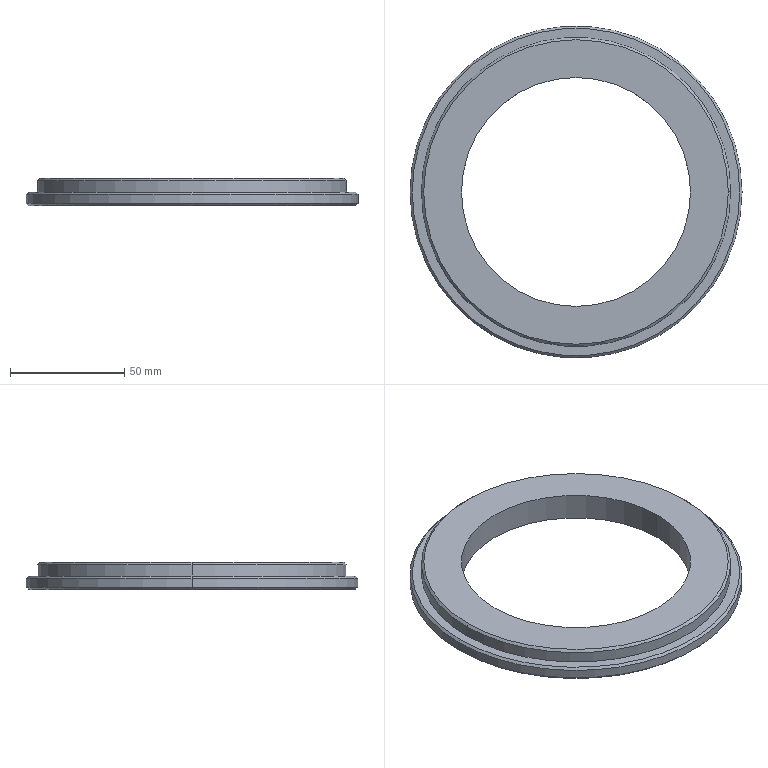Part | SolidWorks | features ICE 2, Chamfer 1, Extrusion 1, HoleWzd 1 | 1 solid | 39 faces | box 145 x 145 x 12 mm | volume 88157 mm3 | cylinder 18 | cone 18 | plane 3 | commonest cylinder face diameters 6.8 x12 100 x2 135 x2 145 x2
STEP:
#1=CARTESIAN_POINT('',(33.4,51.962,8.));
#2=VERTEX_POINT('',#1);
#3=CARTESIAN_POINT('',(26.6,51.962,8.));
#4=VERTEX_POINT('',#3);
#5=CARTESIAN_POINT('',(30.,51.962,8.));
#6=DIRECTION('',(0.,0.,-1.));
#7=DIRECTION('',(-1.,0.,0.));
#8=AXIS2_PLACEMENT_3D('',#5,#6,#7);
#9=CIRCLE('',#8,3.4);
#10=EDGE_CURVE('',#2,#4,#9,.T.);
#11=ORIENTED_EDGE('',*,*,#10,.F.);
#12=CARTESIAN_POINT('',(33.4,51.962,0.));
#13=VERTEX_POINT('',#12);
#14=CARTESIAN_POINT('',(33.4,51.962,0.));
#15=DIRECTION('',(0.,0.,-1.));
#16=VECTOR('',#15,1000.);
#17=LINE('',#14,#16);
#18=EDGE_CURVE('',#2,#13,#17,.T.);
#19=ORIENTED_EDGE('',*,*,#18,.T.);
#20=CARTESIAN_POINT('',(26.6,51.962,0.));
#21=VERTEX_POINT('',#20);
#22=CARTESIAN_POINT('',(30.,51.962,0.));
#23=DIRECTION('',(0.,0.,-1.));
#24=DIRECTION('',(-1.,0.,0.));
#25=AXIS2_PLACEMENT_3D('',#22,#23,#24);
#26=CIRCLE('',#25,3.4);
#27=EDGE_CURVE('',#13,#21,#26,.T.);
#28=ORIENTED_EDGE('',*,*,#27,.T.);
#29=CARTESIAN_POINT('',(26.6,51.962,0.));
#30=DIRECTION('',(0.,0.,-1.));
#31=VECTOR('',#30,1000.);
#32=LINE('',#29,#31);
#33=EDGE_CURVE('',#4,#21,#32,.T.);
#34=ORIENTED_EDGE('',*,*,#33,.F.);
#35=EDGE_LOOP('',(#11,#19,#28,#34));
#36=FACE_OUTER_BOUND('',#35,.T.);
#37=CARTESIAN_POINT('',(30.,51.962,0.));
#38=DIRECTION('',(0.,0.,-1.));
#39=DIRECTION('',(-1.,0.,0.));
#40=AXIS2_PLACEMENT_3D('',#37,#38,#39);
#41=CYLINDRICAL_SURFACE('',#40,3.4);
#42=ADVANCED_FACE('',(#36),#41,.F.);
#43=CARTESIAN_POINT('',(30.,51.962,10.043));
#44=VERTEX_POINT('',#43);
#45=CARTESIAN_POINT('',(26.6,51.962,8.));
#46=DIRECTION('',(-0.8572,0.,-0.515));
#47=VECTOR('',#46,1000.);
#48=LINE('',#45,#47);
#49=EDGE_CURVE('',#44,#4,#48,.T.);
#50=ORIENTED_EDGE('',*,*,#49,.F.);
#51=CARTESIAN_POINT('',(33.4,51.962,8.));
#52=DIRECTION('',(0.8572,0.,-0.515));
#53=VECTOR('',#52,1000.);
#54=LINE('',#51,#53);
#55=EDGE_CURVE('',#44,#2,#54,.T.);
#56=ORIENTED_EDGE('',*,*,#55,.T.);
#57=ORIENTED_EDGE('',*,*,#10,.T.);
#58=EDGE_LOOP('',(#50,#56,#57));
#59=FACE_OUTER_BOUND('',#58,.T.);
#60=CARTESIAN_POINT('',(30.,51.962,8.));
#61=DIRECTION('',(0.,0.,-1.));
#62=DIRECTION('',(-1.,0.,0.));
#63=AXIS2_PLACEMENT_3D('',#60,#61,#62);
#64=CONICAL_SURFACE('',#63,3.4,1.03);
#65=ADVANCED_FACE('',(#59),#64,.F.);
#66=CARTESIAN_POINT('',(-26.6,51.962,8.));
#67=VERTEX_POINT('',#66);
#68=CARTESIAN_POINT('',(-33.4,51.962,8.));
#69=VERTEX_POINT('',#68);
#70=CARTESIAN_POINT('',(-30.,51.962,8.));
#71=DIRECTION('',(0.,0.,-1.));
#72=DIRECTION('',(-1.,0.,0.));
#73=AXIS2_PLACEMENT_3D('',#70,#71,#72);
#74=CIRCLE('',#73,3.4);
#75=EDGE_CURVE('',#67,#69,#74,.T.);
#76=ORIENTED_EDGE('',*,*,#75,.F.);
#77=CARTESIAN_POINT('',(-26.6,51.962,0.));
#78=VERTEX_POINT('',#77);
#79=CARTESIAN_POINT('',(-26.6,51.962,0.));
#80=DIRECTION('',(0.,0.,-1.));
#81=VECTOR('',#80,1000.);
#82=LINE('',#79,#81);
#83=EDGE_CURVE('',#67,#78,#82,.T.);
#84=ORIENTED_EDGE('',*,*,#83,.T.);
#85=CARTESIAN_POINT('',(-33.4,51.962,0.));
#86=VERTEX_POINT('',#85);
#87=CARTESIAN_POINT('',(-30.,51.962,0.));
#88=DIRECTION('',(0.,0.,-1.));
#89=DIRECTION('',(-1.,0.,0.));
#90=AXIS2_PLACEMENT_3D('',#87,#88,#89);
#91=CIRCLE('',#90,3.4);
#92=EDGE_CURVE('',#78,#86,#91,.T.);
#93=ORIENTED_EDGE('',*,*,#92,.T.);
#94=CARTESIAN_POINT('',(-33.4,51.962,0.));
#95=DIRECTION('',(0.,0.,-1.));
#96=VECTOR('',#95,1000.);
#97=LINE('',#94,#96);
#98=EDGE_CURVE('',#69,#86,#97,.T.);
#99=ORIENTED_EDGE('',*,*,#98,.F.);
#100=EDGE_LOOP('',(#76,#84,#93,#99));
#101=FACE_OUTER_BOUND('',#100,.T.);
#102=CARTESIAN_POINT('',(-30.,51.962,0.));
#103=DIRECTION('',(0.,0.,-1.));
#104=DIRECTION('',(-1.,0.,0.));
#105=AXIS2_PLACEMENT_3D('',#102,#103,#104);
#106=CYLINDRICAL_SURFACE('',#105,3.4);
#107=ADVANCED_FACE('',(#101),#106,.F.);
#108=CARTESIAN_POINT('',(-30.,51.962,10.043));
#109=VERTEX_POINT('',#108);
#110=CARTESIAN_POINT('',(-33.4,51.962,8.));
#111=DIRECTION('',(-0.8572,0.,-0.515));
#112=VECTOR('',#111,1000.);
#113=LINE('',#110,#112);
#114=EDGE_CURVE('',#109,#69,#113,.T.);
#115=ORIENTED_EDGE('',*,*,#114,.F.);
#116=CARTESIAN_POINT('',(-26.6,51.962,8.));
#117=DIRECTION('',(0.8572,0.,-0.515));
#118=VECTOR('',#117,1000.);
#119=LINE('',#116,#118);
#120=EDGE_CURVE('',#109,#67,#119,.T.);
#121=ORIENTED_EDGE('',*,*,#120,.T.);
#122=ORIENTED_EDGE('',*,*,#75,.T.);
#123=EDGE_LOOP('',(#115,#121,#122));
#124=FACE_OUTER_BOUND('',#123,.T.);
#125=CARTESIAN_POINT('',(-30.,51.962,8.));
#126=DIRECTION('',(0.,0.,-1.));
#127=DIRECTION('',(-1.,0.,0.));
#128=AXIS2_PLACEMENT_3D('',#125,#126,#127);
#129=CONICAL_SURFACE('',#128,3.4,1.03);
#130=ADVANCED_FACE('',(#124),#129,.F.);
#131=CARTESIAN_POINT('',(-56.6,0.,8.));
#132=VERTEX_POINT('',#131);
#133=CARTESIAN_POINT('',(-63.4,0.,8.));
#134=VERTEX_POINT('',#133);
#135=CARTESIAN_POINT('',(-60.,0.,8.));
#136=DIRECTION('',(0.,0.,-1.));
#137=DIRECTION('',(-1.,0.,0.));
#138=AXIS2_PLACEMENT_3D('',#135,#136,#137);
#139=CIRCLE('',#138,3.4);
#140=EDGE_CURVE('',#132,#134,#139,.T.);
#141=ORIENTED_EDGE('',*,*,#140,.F.);
#142=CARTESIAN_POINT('',(-56.6,0.,0.));
#143=VERTEX_POINT('',#142);
#144=CARTESIAN_POINT('',(-56.6,0.,0.));
#145=DIRECTION('',(0.,0.,-1.));
#146=VECTOR('',#145,1000.);
#147=LINE('',#144,#146);
#148=EDGE_CURVE('',#132,#143,#147,.T.);
#149=ORIENTED_EDGE('',*,*,#148,.T.);
#150=CARTESIAN_POINT('',(-63.4,0.,0.));
#151=VERTEX_POINT('',#150);
#152=CARTESIAN_POINT('',(-60.,0.,0.));
#153=DIRECTION('',(0.,0.,-1.));
#154=DIRECTION('',(-1.,0.,0.));
#155=AXIS2_PLACEMENT_3D('',#152,#153,#154);
#156=CIRCLE('',#155,3.4);
#157=EDGE_CURVE('',#143,#151,#156,.T.);
#158=ORIENTED_EDGE('',*,*,#157,.T.);
#159=CARTESIAN_POINT('',(-63.4,0.,0.));
#160=DIRECTION('',(0.,0.,-1.));
#161=VECTOR('',#160,1000.);
#162=LINE('',#159,#161);
#163=EDGE_CURVE('',#134,#151,#162,.T.);
#164=ORIENTED_EDGE('',*,*,#163,.F.);
#165=EDGE_LOOP('',(#141,#149,#158,#164));
#166=FACE_OUTER_BOUND('',#165,.T.);
#167=CARTESIAN_POINT('',(-60.,0.,0.));
#168=DIRECTION('',(0.,0.,-1.));
#169=DIRECTION('',(-1.,0.,0.));
#170=AXIS2_PLACEMENT_3D('',#167,#168,#169);
#171=CYLINDRICAL_SURFACE('',#170,3.4);
#172=ADVANCED_FACE('',(#166),#171,.F.);
#173=CARTESIAN_POINT('',(-60.,0.,10.043));
#174=VERTEX_POINT('',#173);
#175=CARTESIAN_POINT('',(-63.4,0.,8.));
#176=DIRECTION('',(-0.8572,0.,-0.515));
#177=VECTOR('',#176,1000.);
#178=LINE('',#175,#177);
#179=EDGE_CURVE('',#174,#134,#178,.T.);
#180=ORIENTED_EDGE('',*,*,#179,.F.);
#181=CARTESIAN_POINT('',(-56.6,0.,8.));
#182=DIRECTION('',(0.8572,0.,-0.515));
#183=VECTOR('',#182,1000.);
#184=LINE('',#181,#183);
#185=EDGE_CURVE('',#174,#132,#184,.T.);
#186=ORIENTED_EDGE('',*,*,#185,.T.);
#187=ORIENTED_EDGE('',*,*,#140,.T.);
#188=EDGE_LOOP('',(#180,#186,#187));
#189=FACE_OUTER_BOUND('',#188,.T.);
#190=CARTESIAN_POINT('',(-60.,0.,8.));
#191=DIRECTION('',(0.,0.,-1.));
#192=DIRECTION('',(-1.,0.,0.));
#193=AXIS2_PLACEMENT_3D('',#190,#191,#192);
#194=CONICAL_SURFACE('',#193,3.4,1.03);
#195=ADVANCED_FACE('',(#189),#194,.F.);
#196=CARTESIAN_POINT('',(-26.6,-51.962,8.));
#197=VERTEX_POINT('',#196);
#198=CARTESIAN_POINT('',(-33.4,-51.962,8.));
#199=VERTEX_POINT('',#198);
#200=CARTESIAN_POINT('',(-30.,-51.962,8.));
#201=DIRECTION('',(0.,0.,-1.));
#202=DIRECTION('',(-1.,0.,0.));
#203=AXIS2_PLACEMENT_3D('',#200,#201,#202);
#204=CIRCLE('',#203,3.4);
#205=EDGE_CURVE('',#197,#199,#204,.T.);
#206=ORIENTED_EDGE('',*,*,#205,.F.);
#207=CARTESIAN_POINT('',(-26.6,-51.962,0.));
#208=VERTEX_POINT('',#207);
#209=CARTESIAN_POINT('',(-26.6,-51.962,0.));
#210=DIRECTION('',(0.,0.,-1.));
#211=VECTOR('',#210,1000.);
#212=LINE('',#209,#211);
#213=EDGE_CURVE('',#197,#208,#212,.T.);
#214=ORIENTED_EDGE('',*,*,#213,.T.);
#215=CARTESIAN_POINT('',(-33.4,-51.962,0.));
#216=VERTEX_POINT('',#215);
#217=CARTESIAN_POINT('',(-30.,-51.962,0.));
#218=DIRECTION('',(0.,0.,-1.));
#219=DIRECTION('',(-1.,0.,0.));
#220=AXIS2_PLACEMENT_3D('',#217,#218,#219);
#221=CIRCLE('',#220,3.4);
#222=EDGE_CURVE('',#208,#216,#221,.T.);
#223=ORIENTED_EDGE('',*,*,#222,.T.);
#224=CARTESIAN_POINT('',(-33.4,-51.962,0.));
#225=DIRECTION('',(0.,0.,-1.));
#226=VECTOR('',#225,1000.);
#227=LINE('',#224,#226);
#228=EDGE_CURVE('',#199,#216,#227,.T.);
#229=ORIENTED_EDGE('',*,*,#228,.F.);
#230=EDGE_LOOP('',(#206,#214,#223,#229));
#231=FACE_OUTER_BOUND('',#230,.T.);
#232=CARTESIAN_POINT('',(-30.,-51.962,0.));
#233=DIRECTION('',(0.,0.,-1.));
#234=DIRECTION('',(-1.,0.,0.));
#235=AXIS2_PLACEMENT_3D('',#232,#233,#234);
#236=CYLINDRICAL_SURFACE('',#235,3.4);
#237=ADVANCED_FACE('',(#231),#236,.F.);
#238=CARTESIAN_POINT('',(-30.,-51.962,10.043));
#239=VERTEX_POINT('',#238);
#240=CARTESIAN_POINT('',(-33.4,-51.962,8.));
#241=DIRECTION('',(-0.8572,0.,-0.515));
#242=VECTOR('',#241,1000.);
#243=LINE('',#240,#242);
#244=EDGE_CURVE('',#239,#199,#243,.T.);
#245=ORIENTED_EDGE('',*,*,#244,.F.);
#246=CARTESIAN_POINT('',(-26.6,-51.962,8.));
#247=DIRECTION('',(0.8572,0.,-0.515));
#248=VECTOR('',#247,1000.);
#249=LINE('',#246,#248);
#250=EDGE_CURVE('',#239,#197,#249,.T.);
#251=ORIENTED_EDGE('',*,*,#250,.T.);
#252=ORIENTED_EDGE('',*,*,#205,.T.);
#253=EDGE_LOOP('',(#245,#251,#252));
#254=FACE_OUTER_BOUND('',#253,.T.);
#255=CARTESIAN_POINT('',(-30.,-51.962,8.));
#256=DIRECTION('',(0.,0.,-1.));
#257=DIRECTION('',(-1.,0.,0.));
#258=AXIS2_PLACEMENT_3D('',#255,#256,#257);
#259=CONICAL_SURFACE('',#258,3.4,1.03);
#260=ADVANCED_FACE('',(#254),#259,.F.);
#261=CARTESIAN_POINT('',(33.4,-51.962,8.));
#262=VERTEX_POINT('',#261);
#263=CARTESIAN_POINT('',(26.6,-51.962,8.));
#264=VERTEX_POINT('',#263);
#265=CARTESIAN_POINT('',(30.,-51.962,8.));
#266=DIRECTION('',(0.,0.,-1.));
#267=DIRECTION('',(-1.,0.,0.));
#268=AXIS2_PLACEMENT_3D('',#265,#266,#267);
#269=CIRCLE('',#268,3.4);
#270=EDGE_CURVE('',#262,#264,#269,.T.);
#271=ORIENTED_EDGE('',*,*,#270,.F.);
#272=CARTESIAN_POINT('',(33.4,-51.962,0.));
#273=VERTEX_POINT('',#272);
#274=CARTESIAN_POINT('',(33.4,-51.962,0.));
#275=DIRECTION('',(0.,0.,-1.));
#276=VECTOR('',#275,1000.);
#277=LINE('',#274,#276);
#278=EDGE_CURVE('',#262,#273,#277,.T.);
#279=ORIENTED_EDGE('',*,*,#278,.T.);
#280=CARTESIAN_POINT('',(26.6,-51.962,0.));
#281=VERTEX_POINT('',#280);
#282=CARTESIAN_POINT('',(30.,-51.962,0.));
#283=DIRECTION('',(0.,0.,-1.));
#284=DIRECTION('',(-1.,0.,0.));
#285=AXIS2_PLACEMENT_3D('',#282,#283,#284);
#286=CIRCLE('',#285,3.4);
#287=EDGE_CURVE('',#273,#281,#286,.T.);
#288=ORIENTED_EDGE('',*,*,#287,.T.);
#289=CARTESIAN_POINT('',(26.6,-51.962,0.));
#290=DIRECTION('',(0.,0.,-1.));
#291=VECTOR('',#290,1000.);
#292=LINE('',#289,#291);
#293=EDGE_CURVE('',#264,#281,#292,.T.);
#294=ORIENTED_EDGE('',*,*,#293,.F.);
#295=EDGE_LOOP('',(#271,#279,#288,#294));
#296=FACE_OUTER_BOUND('',#295,.T.);
#297=CARTESIAN_POINT('',(30.,-51.962,0.));
#298=DIRECTION('',(0.,0.,-1.));
#299=DIRECTION('',(-1.,0.,0.));
#300=AXIS2_PLACEMENT_3D('',#297,#298,#299);
#301=CYLINDRICAL_SURFACE('',#300,3.4);
#302=ADVANCED_FACE('',(#296),#301,.F.);
#303=CARTESIAN_POINT('',(30.,-51.962,10.043));
#304=VERTEX_POINT('',#303);
#305=CARTESIAN_POINT('',(26.6,-51.962,8.));
#306=DIRECTION('',(-0.8572,0.,-0.515));
#307=VECTOR('',#306,1000.);
#308=LINE('',#305,#307);
#309=EDGE_CURVE('',#304,#264,#308,.T.);
#310=ORIENTED_EDGE('',*,*,#309,.F.);
#311=CARTESIAN_POINT('',(33.4,-51.962,8.));
#312=DIRECTION('',(0.8572,0.,-0.515));
#313=VECTOR('',#312,1000.);
#314=LINE('',#311,#313);
#315=EDGE_CURVE('',#304,#262,#314,.T.);
#316=ORIENTED_EDGE('',*,*,#315,.T.);
#317=ORIENTED_EDGE('',*,*,#270,.T.);
#318=EDGE_LOOP('',(#310,#316,#317));
#319=FACE_OUTER_BOUND('',#318,.T.);
#320=CARTESIAN_POINT('',(30.,-51.962,8.));
#321=DIRECTION('',(0.,0.,-1.));
#322=DIRECTION('',(-1.,0.,0.));
#323=AXIS2_PLACEMENT_3D('',#320,#321,#322);
#324=CONICAL_SURFACE('',#323,3.4,1.03);
#325=ADVANCED_FACE('',(#319),#324,.F.);
#326=CARTESIAN_POINT('',(63.4,0.,8.));
#327=VERTEX_POINT('',#326);
#328=CARTESIAN_POINT('',(56.6,0.,8.));
#329=VERTEX_POINT('',#328);
#330=CARTESIAN_POINT('',(60.,0.,8.));
#331=DIRECTION('',(0.,0.,-1.));
#332=DIRECTION('',(-1.,0.,0.));
#333=AXIS2_PLACEMENT_3D('',#330,#331,#332);
#334=CIRCLE('',#333,3.4);
#335=EDGE_CURVE('',#327,#329,#334,.T.);
#336=ORIENTED_EDGE('',*,*,#335,.F.);
#337=CARTESIAN_POINT('',(63.4,0.,0.));
#338=VERTEX_POINT('',#337);
#339=CARTESIAN_POINT('',(63.4,0.,0.));
#340=DIRECTION('',(0.,0.,-1.));
#341=VECTOR('',#340,1000.);
#342=LINE('',#339,#341);
#343=EDGE_CURVE('',#327,#338,#342,.T.);
#344=ORIENTED_EDGE('',*,*,#343,.T.);
#345=CARTESIAN_POINT('',(56.6,0.,0.));
#346=VERTEX_POINT('',#345);
#347=CARTESIAN_POINT('',(60.,0.,0.));
#348=DIRECTION('',(0.,0.,-1.));
#349=DIRECTION('',(-1.,0.,0.));
#350=AXIS2_PLACEMENT_3D('',#347,#348,#349);
#351=CIRCLE('',#350,3.4);
#352=EDGE_CURVE('',#338,#346,#351,.T.);
#353=ORIENTED_EDGE('',*,*,#352,.T.);
#354=CARTESIAN_POINT('',(56.6,0.,0.));
#355=DIRECTION('',(0.,0.,-1.));
#356=VECTOR('',#355,1000.);
#357=LINE('',#354,#356);
#358=EDGE_CURVE('',#329,#346,#357,.T.);
#359=ORIENTED_EDGE('',*,*,#358,.F.);
#360=EDGE_LOOP('',(#336,#344,#353,#359));
#361=FACE_OUTER_BOUND('',#360,.T.);
#362=CARTESIAN_POINT('',(60.,0.,0.));
#363=DIRECTION('',(0.,0.,-1.));
#364=DIRECTION('',(-1.,0.,0.));
#365=AXIS2_PLACEMENT_3D('',#362,#363,#364);
#366=CYLINDRICAL_SURFACE('',#365,3.4);
#367=ADVANCED_FACE('',(#361),#366,.F.);
#368=CARTESIAN_POINT('',(60.,0.,10.043));
#369=VERTEX_POINT('',#368);
#370=CARTESIAN_POINT('',(56.6,0.,8.));
#371=DIRECTION('',(-0.8572,0.,-0.515));
#372=VECTOR('',#371,1000.);
#373=LINE('',#370,#372);
#374=EDGE_CURVE('',#369,#329,#373,.T.);
#375=ORIENTED_EDGE('',*,*,#374,.F.);
#376=CARTESIAN_POINT('',(63.4,0.,8.));
#377=DIRECTION('',(0.8572,0.,-0.515));
#378=VECTOR('',#377,1000.);
#379=LINE('',#376,#378);
#380=EDGE_CURVE('',#369,#327,#379,.T.);
#381=ORIENTED_EDGE('',*,*,#380,.T.);
#382=ORIENTED_EDGE('',*,*,#335,.T.);
#383=EDGE_LOOP('',(#375,#381,#382));
#384=FACE_OUTER_BOUND('',#383,.T.);
#385=CARTESIAN_POINT('',(60.,0.,8.));
#386=DIRECTION('',(0.,0.,-1.));
#387=DIRECTION('',(-1.,0.,0.));
#388=AXIS2_PLACEMENT_3D('',#385,#386,#387);
#389=CONICAL_SURFACE('',#388,3.4,1.03);
#390=ADVANCED_FACE('',(#384),#389,.F.);
#391=CARTESIAN_POINT('',(-71.5,0.,0.));
#392=VERTEX_POINT('',#391);
#393=CARTESIAN_POINT('',(71.5,0.,0.));
#394=VERTEX_POINT('',#393);
#395=CARTESIAN_POINT('',(0.,0.,0.));
#396=DIRECTION('',(0.,0.,-1.));
#397=DIRECTION('',(1.,0.,0.));
#398=AXIS2_PLACEMENT_3D('',#395,#396,#397);
#399=CIRCLE('',#398,71.5);
#400=EDGE_CURVE('',#392,#394,#399,.T.);
#401=ORIENTED_EDGE('',*,*,#400,.F.);
#402=CARTESIAN_POINT('',(-72.5,0.,1.));
#403=VERTEX_POINT('',#402);
#404=CARTESIAN_POINT('',(-72.5,0.,1.));
#405=DIRECTION('',(-0.7071,0.,0.7071));
#406=VECTOR('',#405,1000.);
#407=LINE('',#404,#406);
#408=EDGE_CURVE('',#392,#403,#407,.T.);
#409=ORIENTED_EDGE('',*,*,#408,.T.);
#410=CARTESIAN_POINT('',(72.5,0.,1.));
#411=VERTEX_POINT('',#410);
#412=CARTESIAN_POINT('',(0.,0.,1.));
#413=DIRECTION('',(0.,0.,1.));
#414=DIRECTION('',(1.,0.,0.));
#415=AXIS2_PLACEMENT_3D('',#412,#413,#414);
#416=CIRCLE('',#415,72.5);
#417=EDGE_CURVE('',#411,#403,#416,.T.);
#418=ORIENTED_EDGE('',*,*,#417,.F.);
#419=CARTESIAN_POINT('',(72.5,0.,1.));
#420=DIRECTION('',(0.7071,0.,0.7071));
#421=VECTOR('',#420,1000.);
#422=LINE('',#419,#421);
#423=EDGE_CURVE('',#394,#411,#422,.T.);
#424=ORIENTED_EDGE('',*,*,#423,.F.);
#425=EDGE_LOOP('',(#401,#409,#418,#424));
#426=FACE_OUTER_BOUND('',#425,.T.);
#427=CARTESIAN_POINT('',(0.,0.,1.));
#428=DIRECTION('',(0.,0.,1.));
#429=DIRECTION('',(1.,0.,0.));
#430=AXIS2_PLACEMENT_3D('',#427,#428,#429);
#431=CONICAL_SURFACE('',#430,72.5,0.7854);
#432=ADVANCED_FACE('',(#426),#431,.T.);
#433=CARTESIAN_POINT('',(71.5,0.,6.));
#434=VERTEX_POINT('',#433);
#435=CARTESIAN_POINT('',(-71.5,0.,6.));
#436=VERTEX_POINT('',#435);
#437=CARTESIAN_POINT('',(0.,0.,6.));
#438=DIRECTION('',(0.,0.,1.));
#439=DIRECTION('',(1.,0.,0.));
#440=AXIS2_PLACEMENT_3D('',#437,#438,#439);
#441=CIRCLE('',#440,71.5);
#442=EDGE_CURVE('',#434,#436,#441,.T.);
#443=ORIENTED_EDGE('',*,*,#442,.F.);
#444=CARTESIAN_POINT('',(72.5,0.,5.));
#445=VERTEX_POINT('',#444);
#446=CARTESIAN_POINT('',(71.5,0.,6.));
#447=DIRECTION('',(0.7071,0.,-0.7071));
#448=VECTOR('',#447,1000.);
#449=LINE('',#446,#448);
#450=EDGE_CURVE('',#434,#445,#449,.T.);
#451=ORIENTED_EDGE('',*,*,#450,.T.);
#452=CARTESIAN_POINT('',(-72.5,0.,5.));
#453=VERTEX_POINT('',#452);
#454=CARTESIAN_POINT('',(0.,0.,5.));
#455=DIRECTION('',(0.,0.,-1.));
#456=DIRECTION('',(1.,0.,0.));
#457=AXIS2_PLACEMENT_3D('',#454,#455,#456);
#458=CIRCLE('',#457,72.5);
#459=EDGE_CURVE('',#453,#445,#458,.T.);
#460=ORIENTED_EDGE('',*,*,#459,.F.);
#461=CARTESIAN_POINT('',(-71.5,0.,6.));
#462=DIRECTION('',(-0.7071,0.,-0.7071));
#463=VECTOR('',#462,1000.);
#464=LINE('',#461,#463);
#465=EDGE_CURVE('',#436,#453,#464,.T.);
#466=ORIENTED_EDGE('',*,*,#465,.F.);
#467=EDGE_LOOP('',(#443,#451,#460,#466));
#468=FACE_OUTER_BOUND('',#467,.T.);
#469=CARTESIAN_POINT('',(0.,0.,6.));
#470=DIRECTION('',(0.,0.,-1.));
#471=DIRECTION('',(-1.,0.,0.));
#472=AXIS2_PLACEMENT_3D('',#469,#470,#471);
#473=CONICAL_SURFACE('',#472,71.5,0.7854);
#474=ADVANCED_FACE('',(#468),#473,.T.);
#475=CARTESIAN_POINT('',(66.5,0.,12.));
#476=VERTEX_POINT('',#475);
#477=CARTESIAN_POINT('',(-66.5,0.,12.));
#478=VERTEX_POINT('',#477);
#479=CARTESIAN_POINT('',(0.,0.,12.));
#480=DIRECTION('',(0.,0.,1.));
#481=DIRECTION('',(1.,0.,0.));
#482=AXIS2_PLACEMENT_3D('',#479,#480,#481);
#483=CIRCLE('',#482,66.5);
#484=EDGE_CURVE('',#476,#478,#483,.T.);
#485=ORIENTED_EDGE('',*,*,#484,.F.);
#486=CARTESIAN_POINT('',(67.5,0.,11.));
#487=VERTEX_POINT('',#486);
#488=CARTESIAN_POINT('',(66.5,0.,12.));
#489=DIRECTION('',(0.7071,0.,-0.7071));
#490=VECTOR('',#489,1000.);
#491=LINE('',#488,#490);
#492=EDGE_CURVE('',#476,#487,#491,.T.);
#493=ORIENTED_EDGE('',*,*,#492,.T.);
#494=CARTESIAN_POINT('',(-67.5,0.,11.));
#495=VERTEX_POINT('',#494);
#496=CARTESIAN_POINT('',(0.,0.,11.));
#497=DIRECTION('',(0.,0.,-1.));
#498=DIRECTION('',(1.,0.,0.));
#499=AXIS2_PLACEMENT_3D('',#496,#497,#498);
#500=CIRCLE('',#499,67.5);
#501=EDGE_CURVE('',#495,#487,#500,.T.);
#502=ORIENTED_EDGE('',*,*,#501,.F.);
#503=CARTESIAN_POINT('',(-66.5,0.,12.));
#504=DIRECTION('',(-0.7071,0.,-0.7071));
#505=VECTOR('',#504,1000.);
#506=LINE('',#503,#505);
#507=EDGE_CURVE('',#478,#495,#506,.T.);
#508=ORIENTED_EDGE('',*,*,#507,.F.);
#509=EDGE_LOOP('',(#485,#493,#502,#508));
#510=FACE_OUTER_BOUND('',#509,.T.);
#511=CARTESIAN_POINT('',(0.,0.,12.));
#512=DIRECTION('',(0.,0.,-1.));
#513=DIRECTION('',(-1.,0.,0.));
#514=AXIS2_PLACEMENT_3D('',#511,#512,#513);
#515=CONICAL_SURFACE('',#514,66.5,0.7854);
#516=ADVANCED_FACE('',(#510),#515,.T.);
#517=ORIENTED_EDGE('',*,*,#501,.T.);
#518=CARTESIAN_POINT('',(67.5,0.,6.));
#519=VERTEX_POINT('',#518);
#520=CARTESIAN_POINT('',(67.5,0.,12.));
#521=DIRECTION('',(0.,0.,-1.));
#522=VECTOR('',#521,1000.);
#523=LINE('',#520,#522);
#524=EDGE_CURVE('',#487,#519,#523,.T.);
#525=ORIENTED_EDGE('',*,*,#524,.T.);
#526=CARTESIAN_POINT('',(-67.5,0.,6.));
#527=VERTEX_POINT('',#526);
#528=CARTESIAN_POINT('',(0.,0.,6.));
#529=DIRECTION('',(0.,0.,1.));
#530=DIRECTION('',(1.,0.,0.));
#531=AXIS2_PLACEMENT_3D('',#528,#529,#530);
#532=CIRCLE('',#531,67.5);
#533=EDGE_CURVE('',#519,#527,#532,.T.);
#534=ORIENTED_EDGE('',*,*,#533,.T.);
#535=CARTESIAN_POINT('',(-67.5,0.,12.));
#536=DIRECTION('',(0.,0.,-1.));
#537=VECTOR('',#536,1000.);
#538=LINE('',#535,#537);
#539=EDGE_CURVE('',#495,#527,#538,.T.);
#540=ORIENTED_EDGE('',*,*,#539,.F.);
#541=EDGE_LOOP('',(#517,#525,#534,#540));
#542=FACE_OUTER_BOUND('',#541,.T.);
#543=CARTESIAN_POINT('',(0.,0.,12.));
#544=DIRECTION('',(0.,0.,-1.));
#545=DIRECTION('',(-1.,0.,0.));
#546=AXIS2_PLACEMENT_3D('',#543,#544,#545);
#547=CYLINDRICAL_SURFACE('',#546,67.5);
#548=ADVANCED_FACE('',(#542),#547,.T.);
#549=CARTESIAN_POINT('',(-50.,0.,12.));
#550=VERTEX_POINT('',#549);
#551=CARTESIAN_POINT('',(50.,0.,12.));
#552=VERTEX_POINT('',#551);
#553=CARTESIAN_POINT('',(0.,0.,12.));
#554=DIRECTION('',(0.,0.,1.));
#555=DIRECTION('',(1.,0.,0.));
#556=AXIS2_PLACEMENT_3D('',#553,#554,#555);
#557=CIRCLE('',#556,50.);
#558=EDGE_CURVE('',#550,#552,#557,.T.);
#559=ORIENTED_EDGE('',*,*,#558,.T.);
#560=CARTESIAN_POINT('',(50.,0.,0.));
#561=VERTEX_POINT('',#560);
#562=CARTESIAN_POINT('',(50.,0.,6.));
#563=DIRECTION('',(0.,0.,-1.));
#564=VECTOR('',#563,1000.);
#565=LINE('',#562,#564);
#566=EDGE_CURVE('',#552,#561,#565,.T.);
#567=ORIENTED_EDGE('',*,*,#566,.T.);
#568=CARTESIAN_POINT('',(-50.,0.,0.));
#569=VERTEX_POINT('',#568);
#570=CARTESIAN_POINT('',(0.,0.,0.));
#571=DIRECTION('',(0.,0.,1.));
#572=DIRECTION('',(1.,0.,0.));
#573=AXIS2_PLACEMENT_3D('',#570,#571,#572);
#574=CIRCLE('',#573,50.);
#575=EDGE_CURVE('',#569,#561,#574,.T.);
#576=ORIENTED_EDGE('',*,*,#575,.F.);
#577=CARTESIAN_POINT('',(-50.,0.,6.));
#578=DIRECTION('',(0.,0.,-1.));
#579=VECTOR('',#578,1000.);
#580=LINE('',#577,#579);
#581=EDGE_CURVE('',#550,#569,#580,.T.);
#582=ORIENTED_EDGE('',*,*,#581,.F.);
#583=EDGE_LOOP('',(#559,#567,#576,#582));
#584=FACE_OUTER_BOUND('',#583,.T.);
#585=CARTESIAN_POINT('',(0.,0.,6.));
#586=DIRECTION('',(0.,0.,-1.));
#587=DIRECTION('',(-1.,0.,0.));
#588=AXIS2_PLACEMENT_3D('',#585,#586,#587);
#589=CYLINDRICAL_SURFACE('',#588,50.);
#590=ADVANCED_FACE('',(#584),#589,.F.);
#591=ORIENTED_EDGE('',*,*,#459,.T.);
#592=CARTESIAN_POINT('',(72.5,0.,6.));
#593=DIRECTION('',(0.,0.,-1.));
#594=VECTOR('',#593,1000.);
#595=LINE('',#592,#594);
#596=EDGE_CURVE('',#445,#411,#595,.T.);
#597=ORIENTED_EDGE('',*,*,#596,.T.);
#598=ORIENTED_EDGE('',*,*,#417,.T.);
#599=CARTESIAN_POINT('',(-72.5,0.,6.));
#600=DIRECTION('',(0.,0.,-1.));
#601=VECTOR('',#600,1000.);
#602=LINE('',#599,#601);
#603=EDGE_CURVE('',#453,#403,#602,.T.);
#604=ORIENTED_EDGE('',*,*,#603,.F.);
#605=EDGE_LOOP('',(#591,#597,#598,#604));
#606=FACE_OUTER_BOUND('',#605,.T.);
#607=CARTESIAN_POINT('',(0.,0.,6.));
#608=DIRECTION('',(0.,0.,-1.));
#609=DIRECTION('',(-1.,0.,0.));
#610=AXIS2_PLACEMENT_3D('',#607,#608,#609);
#611=CYLINDRICAL_SURFACE('',#610,72.5);
#612=ADVANCED_FACE('',(#606),#611,.T.);
#613=CARTESIAN_POINT('',(0.,0.,6.));
#614=DIRECTION('',(0.,0.,1.));
#615=DIRECTION('',(1.,0.,0.));
#616=AXIS2_PLACEMENT_3D('',#613,#614,#615);
#617=CIRCLE('',#616,71.5);
#618=EDGE_CURVE('',#436,#434,#617,.T.);
#619=ORIENTED_EDGE('',*,*,#618,.T.);
#620=ORIENTED_EDGE('',*,*,#442,.T.);
#621=EDGE_LOOP('',(#619,#620));
#622=FACE_OUTER_BOUND('',#621,.T.);
#623=CARTESIAN_POINT('',(0.,0.,6.));
#624=DIRECTION('',(0.,0.,1.));
#625=DIRECTION('',(1.,0.,0.));
#626=AXIS2_PLACEMENT_3D('',#623,#624,#625);
#627=CIRCLE('',#626,67.5);
#628=EDGE_CURVE('',#527,#519,#627,.T.);
#629=ORIENTED_EDGE('',*,*,#628,.F.);
#630=ORIENTED_EDGE('',*,*,#533,.F.);
#631=EDGE_LOOP('',(#629,#630));
#632=FACE_BOUND('',#631,.T.);
#633=CARTESIAN_POINT('',(0.,0.,6.));
#634=DIRECTION('',(0.,0.,1.));
#635=DIRECTION('',(1.,0.,0.));
#636=AXIS2_PLACEMENT_3D('',#633,#634,#635);
#637=PLANE('',#636);
#638=ADVANCED_FACE('',(#622,#632),#637,.T.);
#639=CARTESIAN_POINT('',(30.,51.962,0.));
#640=DIRECTION('',(0.,0.,-1.));
#641=DIRECTION('',(-1.,0.,0.));
#642=AXIS2_PLACEMENT_3D('',#639,#640,#641);
#643=CIRCLE('',#642,3.4);
#644=EDGE_CURVE('',#21,#13,#643,.T.);
#645=ORIENTED_EDGE('',*,*,#644,.F.);
#646=ORIENTED_EDGE('',*,*,#27,.F.);
#647=EDGE_LOOP('',(#645,#646));
#648=FACE_BOUND('',#647,.T.);
#649=CARTESIAN_POINT('',(-30.,51.962,0.));
#650=DIRECTION('',(0.,0.,-1.));
#651=DIRECTION('',(-1.,0.,0.));
#652=AXIS2_PLACEMENT_3D('',#649,#650,#651);
#653=CIRCLE('',#652,3.4);
#654=EDGE_CURVE('',#86,#78,#653,.T.);
#655=ORIENTED_EDGE('',*,*,#654,.F.);
#656=ORIENTED_EDGE('',*,*,#92,.F.);
#657=EDGE_LOOP('',(#655,#656));
#658=FACE_BOUND('',#657,.T.);
#659=CARTESIAN_POINT('',(-60.,0.,0.));
#660=DIRECTION('',(0.,0.,-1.));
#661=DIRECTION('',(-1.,0.,0.));
#662=AXIS2_PLACEMENT_3D('',#659,#660,#661);
#663=CIRCLE('',#662,3.4);
#664=EDGE_CURVE('',#151,#143,#663,.T.);
#665=ORIENTED_EDGE('',*,*,#664,.F.);
#666=ORIENTED_EDGE('',*,*,#157,.F.);
#667=EDGE_LOOP('',(#665,#666));
#668=FACE_BOUND('',#667,.T.);
#669=CARTESIAN_POINT('',(-30.,-51.962,0.));
#670=DIRECTION('',(0.,0.,-1.));
#671=DIRECTION('',(-1.,0.,0.));
#672=AXIS2_PLACEMENT_3D('',#669,#670,#671);
#673=CIRCLE('',#672,3.4);
#674=EDGE_CURVE('',#216,#208,#673,.T.);
#675=ORIENTED_EDGE('',*,*,#674,.F.);
#676=ORIENTED_EDGE('',*,*,#222,.F.);
#677=EDGE_LOOP('',(#675,#676));
#678=FACE_BOUND('',#677,.T.);
#679=CARTESIAN_POINT('',(30.,-51.962,0.));
#680=DIRECTION('',(0.,0.,-1.));
#681=DIRECTION('',(-1.,0.,0.));
#682=AXIS2_PLACEMENT_3D('',#679,#680,#681);
#683=CIRCLE('',#682,3.4);
#684=EDGE_CURVE('',#281,#273,#683,.T.);
#685=ORIENTED_EDGE('',*,*,#684,.F.);
#686=ORIENTED_EDGE('',*,*,#287,.F.);
#687=EDGE_LOOP('',(#685,#686));
#688=FACE_BOUND('',#687,.T.);
#689=CARTESIAN_POINT('',(60.,0.,0.));
#690=DIRECTION('',(0.,0.,-1.));
#691=DIRECTION('',(-1.,0.,0.));
#692=AXIS2_PLACEMENT_3D('',#689,#690,#691);
#693=CIRCLE('',#692,3.4);
#694=EDGE_CURVE('',#346,#338,#693,.T.);
#695=ORIENTED_EDGE('',*,*,#694,.F.);
#696=ORIENTED_EDGE('',*,*,#352,.F.);
#697=EDGE_LOOP('',(#695,#696));
#698=FACE_BOUND('',#697,.T.);
#699=CARTESIAN_POINT('',(0.,0.,0.));
#700=DIRECTION('',(0.,0.,-1.));
#701=DIRECTION('',(1.,0.,0.));
#702=AXIS2_PLACEMENT_3D('',#699,#700,#701);
#703=CIRCLE('',#702,71.5);
#704=EDGE_CURVE('',#394,#392,#703,.T.);
#705=ORIENTED_EDGE('',*,*,#704,.T.);
#706=ORIENTED_EDGE('',*,*,#400,.T.);
#707=EDGE_LOOP('',(#705,#706));
#708=FACE_OUTER_BOUND('',#707,.T.);
#709=ORIENTED_EDGE('',*,*,#575,.T.);
#710=CARTESIAN_POINT('',(0.,0.,0.));
#711=DIRECTION('',(0.,0.,1.));
#712=DIRECTION('',(1.,0.,0.));
#713=AXIS2_PLACEMENT_3D('',#710,#711,#712);
#714=CIRCLE('',#713,50.);
#715=EDGE_CURVE('',#561,#569,#714,.T.);
#716=ORIENTED_EDGE('',*,*,#715,.T.);
#717=EDGE_LOOP('',(#709,#716));
#718=FACE_BOUND('',#717,.T.);
#719=CARTESIAN_POINT('',(0.,0.,0.));
#720=DIRECTION('',(0.,0.,1.));
#721=DIRECTION('',(1.,0.,0.));
#722=AXIS2_PLACEMENT_3D('',#719,#720,#721);
#723=PLANE('',#722);
#724=ADVANCED_FACE('',(#648,#658,#668,#678,#688,#698,#708,#718),#723,.F.);
#725=ORIENTED_EDGE('',*,*,#596,.F.);
#726=CARTESIAN_POINT('',(0.,0.,5.));
#727=DIRECTION('',(0.,0.,-1.));
#728=DIRECTION('',(1.,0.,0.));
#729=AXIS2_PLACEMENT_3D('',#726,#727,#728);
#730=CIRCLE('',#729,72.5);
#731=EDGE_CURVE('',#445,#453,#730,.T.);
#732=ORIENTED_EDGE('',*,*,#731,.T.);
#733=ORIENTED_EDGE('',*,*,#603,.T.);
#734=CARTESIAN_POINT('',(0.,0.,1.));
#735=DIRECTION('',(0.,0.,1.));
#736=DIRECTION('',(1.,0.,0.));
#737=AXIS2_PLACEMENT_3D('',#734,#735,#736);
#738=CIRCLE('',#737,72.5);
#739=EDGE_CURVE('',#403,#411,#738,.T.);
#740=ORIENTED_EDGE('',*,*,#739,.T.);
#741=EDGE_LOOP('',(#725,#732,#733,#740));
#742=FACE_OUTER_BOUND('',#741,.T.);
#743=CARTESIAN_POINT('',(0.,0.,6.));
#744=DIRECTION('',(0.,0.,-1.));
#745=DIRECTION('',(-1.,0.,0.));
#746=AXIS2_PLACEMENT_3D('',#743,#744,#745);
#747=CYLINDRICAL_SURFACE('',#746,72.5);
#748=ADVANCED_FACE('',(#742),#747,.T.);
#749=ORIENTED_EDGE('',*,*,#566,.F.);
#750=CARTESIAN_POINT('',(0.,0.,12.));
#751=DIRECTION('',(0.,0.,1.));
#752=DIRECTION('',(1.,0.,0.));
#753=AXIS2_PLACEMENT_3D('',#750,#751,#752);
#754=CIRCLE('',#753,50.);
#755=EDGE_CURVE('',#552,#550,#754,.T.);
#756=ORIENTED_EDGE('',*,*,#755,.T.);
#757=ORIENTED_EDGE('',*,*,#581,.T.);
#758=ORIENTED_EDGE('',*,*,#715,.F.);
#759=EDGE_LOOP('',(#749,#756,#757,#758));
#760=FACE_OUTER_BOUND('',#759,.T.);
#761=CARTESIAN_POINT('',(0.,0.,6.));
#762=DIRECTION('',(0.,0.,-1.));
#763=DIRECTION('',(-1.,0.,0.));
#764=AXIS2_PLACEMENT_3D('',#761,#762,#763);
#765=CYLINDRICAL_SURFACE('',#764,50.);
#766=ADVANCED_FACE('',(#760),#765,.F.);
#767=CARTESIAN_POINT('',(0.,0.,12.));
#768=DIRECTION('',(0.,0.,1.));
#769=DIRECTION('',(1.,0.,0.));
#770=AXIS2_PLACEMENT_3D('',#767,#768,#769);
#771=CIRCLE('',#770,66.5);
#772=EDGE_CURVE('',#478,#476,#771,.T.);
#773=ORIENTED_EDGE('',*,*,#772,.T.);
#774=ORIENTED_EDGE('',*,*,#484,.T.);
#775=EDGE_LOOP('',(#773,#774));
#776=FACE_OUTER_BOUND('',#775,.T.);
#777=ORIENTED_EDGE('',*,*,#558,.F.);
#778=ORIENTED_EDGE('',*,*,#755,.F.);
#779=EDGE_LOOP('',(#777,#778));
#780=FACE_BOUND('',#779,.T.);
#781=CARTESIAN_POINT('',(0.,0.,12.));
#782=DIRECTION('',(0.,0.,1.));
#783=DIRECTION('',(1.,0.,0.));
#784=AXIS2_PLACEMENT_3D('',#781,#782,#783);
#785=PLANE('',#784);
#786=ADVANCED_FACE('',(#776,#780),#785,.T.);
#787=ORIENTED_EDGE('',*,*,#524,.F.);
#788=CARTESIAN_POINT('',(0.,0.,11.));
#789=DIRECTION('',(0.,0.,-1.));
#790=DIRECTION('',(1.,0.,0.));
#791=AXIS2_PLACEMENT_3D('',#788,#789,#790);
#792=CIRCLE('',#791,67.5);
#793=EDGE_CURVE('',#487,#495,#792,.T.);
#794=ORIENTED_EDGE('',*,*,#793,.T.);
#795=ORIENTED_EDGE('',*,*,#539,.T.);
#796=ORIENTED_EDGE('',*,*,#628,.T.);
#797=EDGE_LOOP('',(#787,#794,#795,#796));
#798=FACE_OUTER_BOUND('',#797,.T.);
#799=CARTESIAN_POINT('',(0.,0.,12.));
#800=DIRECTION('',(0.,0.,-1.));
#801=DIRECTION('',(-1.,0.,0.));
#802=AXIS2_PLACEMENT_3D('',#799,#800,#801);
#803=CYLINDRICAL_SURFACE('',#802,67.5);
#804=ADVANCED_FACE('',(#798),#803,.T.);
#805=ORIENTED_EDGE('',*,*,#492,.F.);
#806=ORIENTED_EDGE('',*,*,#772,.F.);
#807=ORIENTED_EDGE('',*,*,#507,.T.);
#808=ORIENTED_EDGE('',*,*,#793,.F.);
#809=EDGE_LOOP('',(#805,#806,#807,#808));
#810=FACE_OUTER_BOUND('',#809,.T.);
#811=CARTESIAN_POINT('',(0.,0.,12.));
#812=DIRECTION('',(0.,0.,-1.));
#813=DIRECTION('',(-1.,0.,0.));
#814=AXIS2_PLACEMENT_3D('',#811,#812,#813);
#815=CONICAL_SURFACE('',#814,66.5,0.7854);
#816=ADVANCED_FACE('',(#810),#815,.T.);
#817=ORIENTED_EDGE('',*,*,#450,.F.);
#818=ORIENTED_EDGE('',*,*,#618,.F.);
#819=ORIENTED_EDGE('',*,*,#465,.T.);
#820=ORIENTED_EDGE('',*,*,#731,.F.);
#821=EDGE_LOOP('',(#817,#818,#819,#820));
#822=FACE_OUTER_BOUND('',#821,.T.);
#823=CARTESIAN_POINT('',(0.,0.,6.));
#824=DIRECTION('',(0.,0.,-1.));
#825=DIRECTION('',(-1.,0.,0.));
#826=AXIS2_PLACEMENT_3D('',#823,#824,#825);
#827=CONICAL_SURFACE('',#826,71.5,0.7854);
#828=ADVANCED_FACE('',(#822),#827,.T.);
#829=ORIENTED_EDGE('',*,*,#408,.F.);
#830=ORIENTED_EDGE('',*,*,#704,.F.);
#831=ORIENTED_EDGE('',*,*,#423,.T.);
#832=ORIENTED_EDGE('',*,*,#739,.F.);
#833=EDGE_LOOP('',(#829,#830,#831,#832));
#834=FACE_OUTER_BOUND('',#833,.T.);
#835=CARTESIAN_POINT('',(0.,0.,1.));
#836=DIRECTION('',(0.,0.,1.));
#837=DIRECTION('',(1.,0.,0.));
#838=AXIS2_PLACEMENT_3D('',#835,#836,#837);
#839=CONICAL_SURFACE('',#838,72.5,0.7854);
#840=ADVANCED_FACE('',(#834),#839,.T.);
#841=ORIENTED_EDGE('',*,*,#380,.F.);
#842=ORIENTED_EDGE('',*,*,#374,.T.);
#843=CARTESIAN_POINT('',(60.,0.,8.));
#844=DIRECTION('',(0.,0.,-1.));
#845=DIRECTION('',(-1.,0.,0.));
#846=AXIS2_PLACEMENT_3D('',#843,#844,#845);
#847=CIRCLE('',#846,3.4);
#848=EDGE_CURVE('',#329,#327,#847,.T.);
#849=ORIENTED_EDGE('',*,*,#848,.T.);
#850=EDGE_LOOP('',(#841,#842,#849));
#851=FACE_OUTER_BOUND('',#850,.T.);
#852=CARTESIAN_POINT('',(60.,0.,8.));
#853=DIRECTION('',(0.,0.,-1.));
#854=DIRECTION('',(-1.,0.,0.));
#855=AXIS2_PLACEMENT_3D('',#852,#853,#854);
#856=CONICAL_SURFACE('',#855,3.4,1.03);
#857=ADVANCED_FACE('',(#851),#856,.F.);
#858=ORIENTED_EDGE('',*,*,#343,.F.);
#859=ORIENTED_EDGE('',*,*,#848,.F.);
#860=ORIENTED_EDGE('',*,*,#358,.T.);
#861=ORIENTED_EDGE('',*,*,#694,.T.);
#862=EDGE_LOOP('',(#858,#859,#860,#861));
#863=FACE_OUTER_BOUND('',#862,.T.);
#864=CARTESIAN_POINT('',(60.,0.,0.));
#865=DIRECTION('',(0.,0.,-1.));
#866=DIRECTION('',(-1.,0.,0.));
#867=AXIS2_PLACEMENT_3D('',#864,#865,#866);
#868=CYLINDRICAL_SURFACE('',#867,3.4);
#869=ADVANCED_FACE('',(#863),#868,.F.);
#870=ORIENTED_EDGE('',*,*,#315,.F.);
#871=ORIENTED_EDGE('',*,*,#309,.T.);
#872=CARTESIAN_POINT('',(30.,-51.962,8.));
#873=DIRECTION('',(0.,0.,-1.));
#874=DIRECTION('',(-1.,0.,0.));
#875=AXIS2_PLACEMENT_3D('',#872,#873,#874);
#876=CIRCLE('',#875,3.4);
#877=EDGE_CURVE('',#264,#262,#876,.T.);
#878=ORIENTED_EDGE('',*,*,#877,.T.);
#879=EDGE_LOOP('',(#870,#871,#878));
#880=FACE_OUTER_BOUND('',#879,.T.);
#881=CARTESIAN_POINT('',(30.,-51.962,8.));
#882=DIRECTION('',(0.,0.,-1.));
#883=DIRECTION('',(-1.,0.,0.));
#884=AXIS2_PLACEMENT_3D('',#881,#882,#883);
#885=CONICAL_SURFACE('',#884,3.4,1.03);
#886=ADVANCED_FACE('',(#880),#885,.F.);
#887=ORIENTED_EDGE('',*,*,#278,.F.);
#888=ORIENTED_EDGE('',*,*,#877,.F.);
#889=ORIENTED_EDGE('',*,*,#293,.T.);
#890=ORIENTED_EDGE('',*,*,#684,.T.);
#891=EDGE_LOOP('',(#887,#888,#889,#890));
#892=FACE_OUTER_BOUND('',#891,.T.);
#893=CARTESIAN_POINT('',(30.,-51.962,0.));
#894=DIRECTION('',(0.,0.,-1.));
#895=DIRECTION('',(-1.,0.,0.));
#896=AXIS2_PLACEMENT_3D('',#893,#894,#895);
#897=CYLINDRICAL_SURFACE('',#896,3.4);
#898=ADVANCED_FACE('',(#892),#897,.F.);
#899=ORIENTED_EDGE('',*,*,#250,.F.);
#900=ORIENTED_EDGE('',*,*,#244,.T.);
#901=CARTESIAN_POINT('',(-30.,-51.962,8.));
#902=DIRECTION('',(0.,0.,-1.));
#903=DIRECTION('',(-1.,0.,0.));
#904=AXIS2_PLACEMENT_3D('',#901,#902,#903);
#905=CIRCLE('',#904,3.4);
#906=EDGE_CURVE('',#199,#197,#905,.T.);
#907=ORIENTED_EDGE('',*,*,#906,.T.);
#908=EDGE_LOOP('',(#899,#900,#907));
#909=FACE_OUTER_BOUND('',#908,.T.);
#910=CARTESIAN_POINT('',(-30.,-51.962,8.));
#911=DIRECTION('',(0.,0.,-1.));
#912=DIRECTION('',(-1.,0.,0.));
#913=AXIS2_PLACEMENT_3D('',#910,#911,#912);
#914=CONICAL_SURFACE('',#913,3.4,1.03);
#915=ADVANCED_FACE('',(#909),#914,.F.);
#916=ORIENTED_EDGE('',*,*,#213,.F.);
#917=ORIENTED_EDGE('',*,*,#906,.F.);
#918=ORIENTED_EDGE('',*,*,#228,.T.);
#919=ORIENTED_EDGE('',*,*,#674,.T.);
#920=EDGE_LOOP('',(#916,#917,#918,#919));
#921=FACE_OUTER_BOUND('',#920,.T.);
#922=CARTESIAN_POINT('',(-30.,-51.962,0.));
#923=DIRECTION('',(0.,0.,-1.));
#924=DIRECTION('',(-1.,0.,0.));
#925=AXIS2_PLACEMENT_3D('',#922,#923,#924);
#926=CYLINDRICAL_SURFACE('',#925,3.4);
#927=ADVANCED_FACE('',(#921),#926,.F.);
#928=ORIENTED_EDGE('',*,*,#185,.F.);
#929=ORIENTED_EDGE('',*,*,#179,.T.);
#930=CARTESIAN_POINT('',(-60.,0.,8.));
#931=DIRECTION('',(0.,0.,-1.));
#932=DIRECTION('',(-1.,0.,0.));
#933=AXIS2_PLACEMENT_3D('',#930,#931,#932);
#934=CIRCLE('',#933,3.4);
#935=EDGE_CURVE('',#134,#132,#934,.T.);
#936=ORIENTED_EDGE('',*,*,#935,.T.);
#937=EDGE_LOOP('',(#928,#929,#936));
#938=FACE_OUTER_BOUND('',#937,.T.);
#939=CARTESIAN_POINT('',(-60.,0.,8.));
#940=DIRECTION('',(0.,0.,-1.));
#941=DIRECTION('',(-1.,0.,0.));
#942=AXIS2_PLACEMENT_3D('',#939,#940,#941);
#943=CONICAL_SURFACE('',#942,3.4,1.03);
#944=ADVANCED_FACE('',(#938),#943,.F.);
#945=ORIENTED_EDGE('',*,*,#148,.F.);
#946=ORIENTED_EDGE('',*,*,#935,.F.);
#947=ORIENTED_EDGE('',*,*,#163,.T.);
#948=ORIENTED_EDGE('',*,*,#664,.T.);
#949=EDGE_LOOP('',(#945,#946,#947,#948));
#950=FACE_OUTER_BOUND('',#949,.T.);
#951=CARTESIAN_POINT('',(-60.,0.,0.));
#952=DIRECTION('',(0.,0.,-1.));
#953=DIRECTION('',(-1.,0.,0.));
#954=AXIS2_PLACEMENT_3D('',#951,#952,#953);
#955=CYLINDRICAL_SURFACE('',#954,3.4);
#956=ADVANCED_FACE('',(#950),#955,.F.);
#957=ORIENTED_EDGE('',*,*,#120,.F.);
#958=ORIENTED_EDGE('',*,*,#114,.T.);
#959=CARTESIAN_POINT('',(-30.,51.962,8.));
#960=DIRECTION('',(0.,0.,-1.));
#961=DIRECTION('',(-1.,0.,0.));
#962=AXIS2_PLACEMENT_3D('',#959,#960,#961);
#963=CIRCLE('',#962,3.4);
#964=EDGE_CURVE('',#69,#67,#963,.T.);
#965=ORIENTED_EDGE('',*,*,#964,.T.);
#966=EDGE_LOOP('',(#957,#958,#965));
#967=FACE_OUTER_BOUND('',#966,.T.);
#968=CARTESIAN_POINT('',(-30.,51.962,8.));
#969=DIRECTION('',(0.,0.,-1.));
#970=DIRECTION('',(-1.,0.,0.));
#971=AXIS2_PLACEMENT_3D('',#968,#969,#970);
#972=CONICAL_SURFACE('',#971,3.4,1.03);
#973=ADVANCED_FACE('',(#967),#972,.F.);
#974=ORIENTED_EDGE('',*,*,#83,.F.);
#975=ORIENTED_EDGE('',*,*,#964,.F.);
#976=ORIENTED_EDGE('',*,*,#98,.T.);
#977=ORIENTED_EDGE('',*,*,#654,.T.);
#978=EDGE_LOOP('',(#974,#975,#976,#977));
#979=FACE_OUTER_BOUND('',#978,.T.);
#980=CARTESIAN_POINT('',(-30.,51.962,0.));
#981=DIRECTION('',(0.,0.,-1.));
#982=DIRECTION('',(-1.,0.,0.));
#983=AXIS2_PLACEMENT_3D('',#980,#981,#982);
#984=CYLINDRICAL_SURFACE('',#983,3.4);
#985=ADVANCED_FACE('',(#979),#984,.F.);
#986=ORIENTED_EDGE('',*,*,#55,.F.);
#987=ORIENTED_EDGE('',*,*,#49,.T.);
#988=CARTESIAN_POINT('',(30.,51.962,8.));
#989=DIRECTION('',(0.,0.,-1.));
#990=DIRECTION('',(-1.,0.,0.));
#991=AXIS2_PLACEMENT_3D('',#988,#989,#990);
#992=CIRCLE('',#991,3.4);
#993=EDGE_CURVE('',#4,#2,#992,.T.);
#994=ORIENTED_EDGE('',*,*,#993,.T.);
#995=EDGE_LOOP('',(#986,#987,#994));
#996=FACE_OUTER_BOUND('',#995,.T.);
#997=CARTESIAN_POINT('',(30.,51.962,8.));
#998=DIRECTION('',(0.,0.,-1.));
#999=DIRECTION('',(-1.,0.,0.));
#1000=AXIS2_PLACEMENT_3D('',#997,#998,#999);
#1001=CONICAL_SURFACE('',#1000,3.4,1.03);
#1002=ADVANCED_FACE('',(#996),#1001,.F.);
#1003=ORIENTED_EDGE('',*,*,#18,.F.);
#1004=ORIENTED_EDGE('',*,*,#993,.F.);
#1005=ORIENTED_EDGE('',*,*,#33,.T.);
#1006=ORIENTED_EDGE('',*,*,#644,.T.);
#1007=EDGE_LOOP('',(#1003,#1004,#1005,#1006));
#1008=FACE_OUTER_BOUND('',#1007,.T.);
#1009=CARTESIAN_POINT('',(30.,51.962,0.));
#1010=DIRECTION('',(0.,0.,-1.));
#1011=DIRECTION('',(-1.,0.,0.));
#1012=AXIS2_PLACEMENT_3D('',#1009,#1010,#1011);
#1013=CYLINDRICAL_SURFACE('',#1012,3.4);
#1014=ADVANCED_FACE('',(#1008),#1013,.F.);
#1015=CLOSED_SHELL('',(#42,#65,#107,#130,#172,#195,#237,#260,#302,#325,#367,#390,#432,#474,#516,#548,#590,#612,#638,#724,#748,#766,#786,#804,#816,#828,#840,#857,#869,#886,#898,#915,#927,#944,#956,#973,#985,#1002,#1014));
#1016=MANIFOLD_SOLID_BREP('',#1015);
#1017=CARTESIAN_POINT('',(0.,0.,0.));
#1018=DIRECTION('',(0.,0.,1.));
#1019=DIRECTION('',(1.,0.,0.));
#1020=AXIS2_PLACEMENT_3D('',#1017,#1018,#1019);
#1021=(LENGTH_UNIT()NAMED_UNIT(*)SI_UNIT(.MILLI.,.METRE.));
#1022=UNCERTAINTY_MEASURE_WITH_UNIT(LENGTH_MEASURE(0.00001),#1021,'','');
#1023=(NAMED_UNIT(*)PLANE_ANGLE_UNIT()SI_UNIT($,.RADIAN.));
#1024=(NAMED_UNIT(*)SI_UNIT($,.STERADIAN.)SOLID_ANGLE_UNIT());
#1025=(GEOMETRIC_REPRESENTATION_CONTEXT(3)GLOBAL_UNCERTAINTY_ASSIGNED_CONTEXT((#1022))GLOBAL_UNIT_ASSIGNED_CONTEXT((#1021,#1023,#1024))REPRESENTATION_CONTEXT('',''));
#1026=ADVANCED_BREP_SHAPE_REPRESENTATION('',(#1016,#1020),#1025);